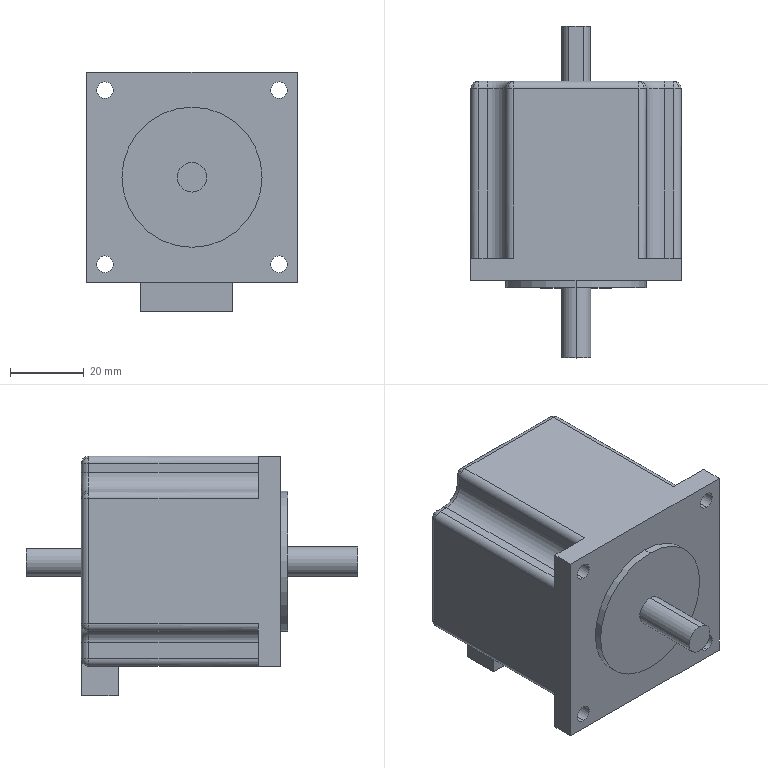Part | NX | features BREP 1 | 1 solid | 85 faces | box 57 x 90 x 65 mm | volume 164072 mm3 | cylinder 39 | plane 26 | sphere 16 | torus 4 | commonest cylinder face diameters 4 x21 4.5 x8 8 x4 10 x3 38 x2 6 x1